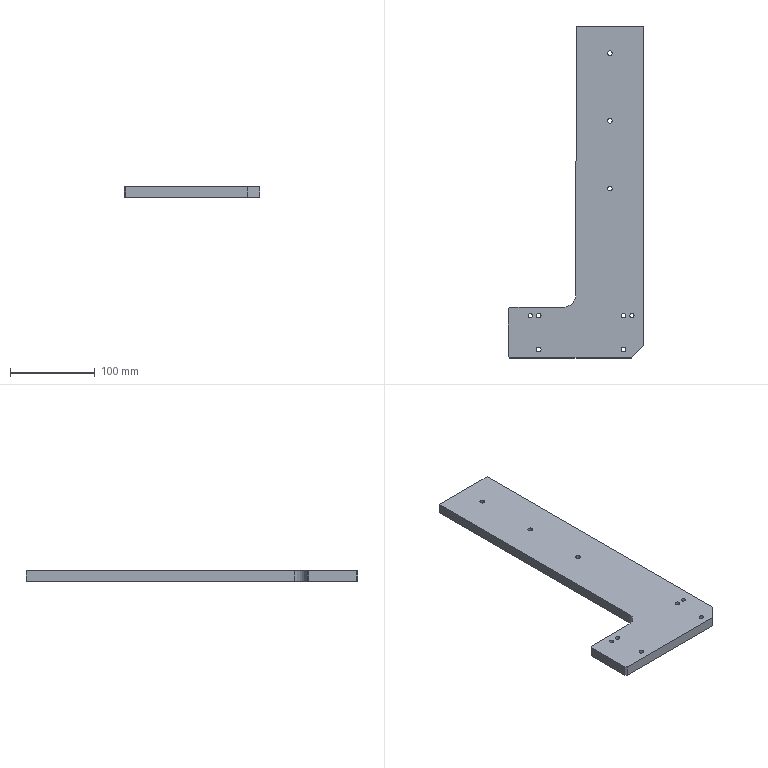Part | STEP file | PN_0045 Mount electronic clip mounting plate 6 | 1 solid | 63 faces | box 160 x 392 x 12 mm | volume 427849 mm3 | cylinder 39 | plane 18 | cone 6 | commonest cylinder face diameters 5.5 x14 10 x14 4.2 x6 5 x4 30 x1